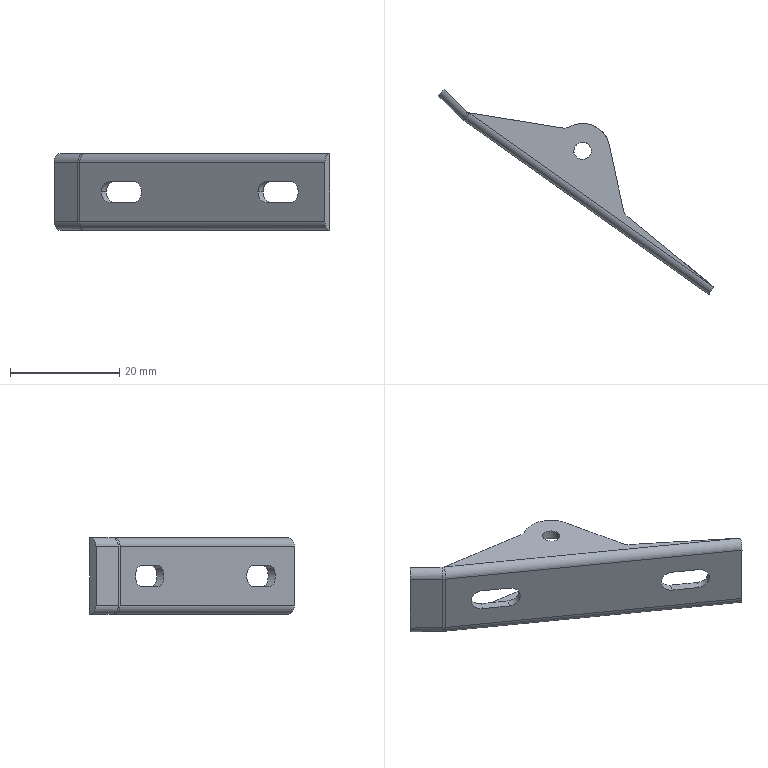Part | SolidWorks | features BaseBody 1 | 1 solid | 50 faces | box 50.411 x 37.401 x 14 mm | volume 1906 mm3 | cylinder 22 | plane 20 | spline 8 | commonest cylinder face diameters 4 x10 3.2 x8 2 x2 10 x2